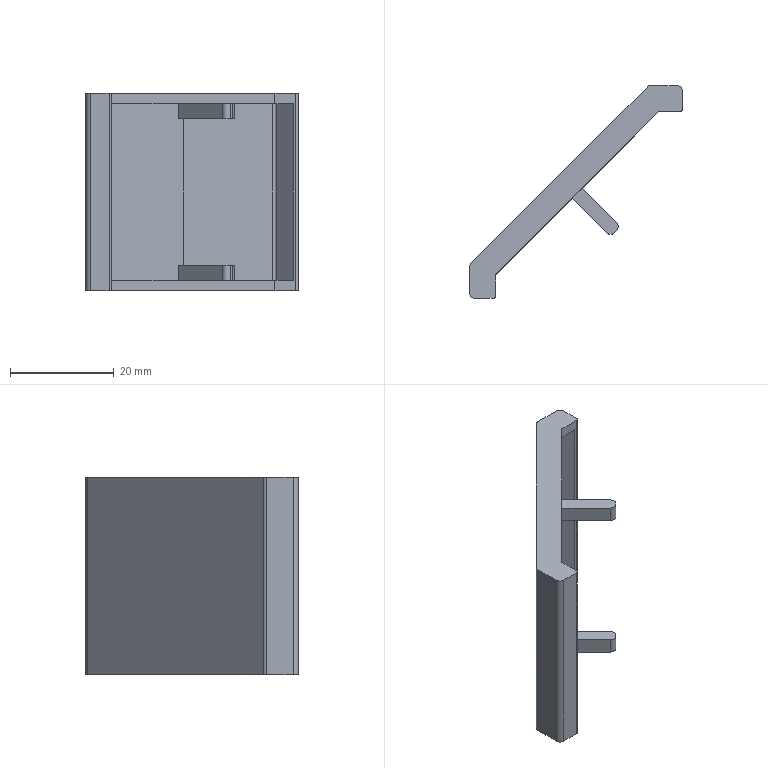Part | SolidWorks | features BaseBody 1 | 1 solid | 42 faces | box 41 x 41 x 38 mm | volume 6489 mm3 | plane 29 | cylinder 13 | commonest cylinder face diameters 2 x9 1 x4
STEP:
#1=CARTESIAN_POINT('',(11.11,-10.616,-17.));
#2=VERTEX_POINT('',#1);
#3=CARTESIAN_POINT('',(11.403,-9.909,-17.));
#4=VERTEX_POINT('',#3);
#5=CARTESIAN_POINT('',(10.403,-9.909,-17.));
#6=DIRECTION('',(0.,0.,1.));
#7=DIRECTION('',(1.,0.,0.));
#8=AXIS2_PLACEMENT_3D('',#5,#6,#7);
#9=CIRCLE('',#8,1.);
#10=EDGE_CURVE('',#2,#4,#9,.T.);
#11=ORIENTED_EDGE('',*,*,#10,.T.);
#12=CARTESIAN_POINT('',(11.403,-9.909,-14.1));
#13=VERTEX_POINT('',#12);
#14=CARTESIAN_POINT('',(11.403,-9.909,-14.1));
#15=DIRECTION('',(0.,0.,1.));
#16=VECTOR('',#15,1000.);
#17=LINE('',#14,#16);
#18=EDGE_CURVE('',#4,#13,#17,.T.);
#19=ORIENTED_EDGE('',*,*,#18,.T.);
#20=CARTESIAN_POINT('',(11.11,-10.616,-14.1));
#21=VERTEX_POINT('',#20);
#22=CARTESIAN_POINT('',(10.403,-9.909,-14.1));
#23=DIRECTION('',(0.,0.,1.));
#24=DIRECTION('',(1.,0.,0.));
#25=AXIS2_PLACEMENT_3D('',#22,#23,#24);
#26=CIRCLE('',#25,1.);
#27=EDGE_CURVE('',#21,#13,#26,.T.);
#28=ORIENTED_EDGE('',*,*,#27,.F.);
#29=CARTESIAN_POINT('',(11.11,-10.616,-14.1));
#30=DIRECTION('',(0.,0.,-1.));
#31=VECTOR('',#30,1000.);
#32=LINE('',#29,#31);
#33=EDGE_CURVE('',#21,#2,#32,.T.);
#34=ORIENTED_EDGE('',*,*,#33,.T.);
#35=EDGE_LOOP('',(#11,#19,#28,#34));
#36=FACE_OUTER_BOUND('',#35,.T.);
#37=CARTESIAN_POINT('',(10.403,-9.909,-14.1));
#38=DIRECTION('',(0.,0.,1.));
#39=DIRECTION('',(1.,0.,0.));
#40=AXIS2_PLACEMENT_3D('',#37,#38,#39);
#41=CYLINDRICAL_SURFACE('',#40,1.);
#42=ADVANCED_FACE('',(#36),#41,.T.);
#43=CARTESIAN_POINT('',(-16.957,-16.957,19.));
#44=VERTEX_POINT('',#43);
#45=CARTESIAN_POINT('',(-16.957,-16.957,-19.));
#46=VERTEX_POINT('',#45);
#47=CARTESIAN_POINT('',(-16.957,-16.957,19.));
#48=DIRECTION('',(0.,0.,-1.));
#49=VECTOR('',#48,1000.);
#50=LINE('',#47,#49);
#51=EDGE_CURVE('',#44,#46,#50,.T.);
#52=ORIENTED_EDGE('',*,*,#51,.F.);
#53=CARTESIAN_POINT('',(16.957,16.957,19.));
#54=VERTEX_POINT('',#53);
#55=CARTESIAN_POINT('',(16.957,16.957,19.));
#56=DIRECTION('',(-0.7071,-0.7071,0.));
#57=VECTOR('',#56,1000.);
#58=LINE('',#55,#57);
#59=EDGE_CURVE('',#54,#44,#58,.T.);
#60=ORIENTED_EDGE('',*,*,#59,.F.);
#61=CARTESIAN_POINT('',(16.957,16.957,-19.));
#62=VERTEX_POINT('',#61);
#63=CARTESIAN_POINT('',(16.957,16.957,19.));
#64=DIRECTION('',(0.,0.,1.));
#65=VECTOR('',#64,1000.);
#66=LINE('',#63,#65);
#67=EDGE_CURVE('',#62,#54,#66,.T.);
#68=ORIENTED_EDGE('',*,*,#67,.F.);
#69=CARTESIAN_POINT('',(16.957,16.957,-19.));
#70=DIRECTION('',(0.7071,0.7071,0.));
#71=VECTOR('',#70,1000.);
#72=LINE('',#69,#71);
#73=EDGE_CURVE('',#46,#62,#72,.T.);
#74=ORIENTED_EDGE('',*,*,#73,.F.);
#75=EDGE_LOOP('',(#52,#60,#68,#74));
#76=FACE_OUTER_BOUND('',#75,.T.);
#77=CARTESIAN_POINT('',(16.957,16.957,19.));
#78=DIRECTION('',(0.7071,-0.7071,0.));
#79=DIRECTION('',(0.7071,0.7071,0.));
#80=AXIS2_PLACEMENT_3D('',#77,#78,#79);
#81=PLANE('',#80);
#82=ADVANCED_FACE('',(#76),#81,.F.);
#83=CARTESIAN_POINT('',(-17.25,-17.664,-19.));
#84=VERTEX_POINT('',#83);
#85=CARTESIAN_POINT('',(-16.25,-17.664,-19.));
#86=DIRECTION('',(0.,0.,1.));
#87=DIRECTION('',(1.,0.,0.));
#88=AXIS2_PLACEMENT_3D('',#85,#86,#87);
#89=CIRCLE('',#88,1.);
#90=EDGE_CURVE('',#46,#84,#89,.T.);
#91=ORIENTED_EDGE('',*,*,#90,.F.);
#92=ORIENTED_EDGE('',*,*,#73,.T.);
#93=CARTESIAN_POINT('',(17.664,17.25,-19.));
#94=VERTEX_POINT('',#93);
#95=CARTESIAN_POINT('',(17.664,16.25,-19.));
#96=DIRECTION('',(0.,0.,1.));
#97=DIRECTION('',(1.,0.,0.));
#98=AXIS2_PLACEMENT_3D('',#95,#96,#97);
#99=CIRCLE('',#98,1.);
#100=EDGE_CURVE('',#94,#62,#99,.T.);
#101=ORIENTED_EDGE('',*,*,#100,.F.);
#102=CARTESIAN_POINT('',(22.75,17.25,-19.));
#103=VERTEX_POINT('',#102);
#104=CARTESIAN_POINT('',(-16.25,17.25,-19.));
#105=DIRECTION('',(-1.,0.,0.));
#106=VECTOR('',#105,1000.);
#107=LINE('',#104,#106);
#108=EDGE_CURVE('',#103,#94,#107,.T.);
#109=ORIENTED_EDGE('',*,*,#108,.F.);
#110=CARTESIAN_POINT('',(23.75,16.25,-19.));
#111=VERTEX_POINT('',#110);
#112=CARTESIAN_POINT('',(22.75,16.25,-19.));
#113=DIRECTION('',(0.,0.,1.));
#114=DIRECTION('',(1.,0.,0.));
#115=AXIS2_PLACEMENT_3D('',#112,#113,#114);
#116=CIRCLE('',#115,1.);
#117=EDGE_CURVE('',#111,#103,#116,.T.);
#118=ORIENTED_EDGE('',*,*,#117,.F.);
#119=CARTESIAN_POINT('',(23.75,12.75,-19.));
#120=VERTEX_POINT('',#119);
#121=CARTESIAN_POINT('',(23.75,-22.75,-19.));
#122=DIRECTION('',(0.,1.,0.));
#123=VECTOR('',#122,1000.);
#124=LINE('',#121,#123);
#125=EDGE_CURVE('',#120,#111,#124,.T.);
#126=ORIENTED_EDGE('',*,*,#125,.F.);
#127=CARTESIAN_POINT('',(23.25,12.25,-19.));
#128=VERTEX_POINT('',#127);
#129=CARTESIAN_POINT('',(23.25,12.75,-19.));
#130=DIRECTION('',(0.,0.,1.));
#131=DIRECTION('',(1.,0.,0.));
#132=AXIS2_PLACEMENT_3D('',#129,#130,#131);
#133=CIRCLE('',#132,0.5);
#134=EDGE_CURVE('',#128,#120,#133,.T.);
#135=ORIENTED_EDGE('',*,*,#134,.F.);
#136=CARTESIAN_POINT('',(19.25,12.25,-19.));
#137=VERTEX_POINT('',#136);
#138=CARTESIAN_POINT('',(-16.25,12.25,-19.));
#139=DIRECTION('',(1.,0.,0.));
#140=VECTOR('',#139,1000.);
#141=LINE('',#138,#140);
#142=EDGE_CURVE('',#137,#128,#141,.T.);
#143=ORIENTED_EDGE('',*,*,#142,.F.);
#144=CARTESIAN_POINT('',(-12.25,-19.25,-19.));
#145=VERTEX_POINT('',#144);
#146=CARTESIAN_POINT('',(-12.25,-19.25,-19.));
#147=DIRECTION('',(0.7071,0.7071,0.));
#148=VECTOR('',#147,1000.);
#149=LINE('',#146,#148);
#150=EDGE_CURVE('',#145,#137,#149,.T.);
#151=ORIENTED_EDGE('',*,*,#150,.F.);
#152=CARTESIAN_POINT('',(-12.25,-23.25,-19.));
#153=VERTEX_POINT('',#152);
#154=CARTESIAN_POINT('',(-12.25,-22.75,-19.));
#155=DIRECTION('',(0.,1.,0.));
#156=VECTOR('',#155,1000.);
#157=LINE('',#154,#156);
#158=EDGE_CURVE('',#153,#145,#157,.T.);
#159=ORIENTED_EDGE('',*,*,#158,.F.);
#160=CARTESIAN_POINT('',(-12.75,-23.75,-19.));
#161=VERTEX_POINT('',#160);
#162=CARTESIAN_POINT('',(-12.75,-23.25,-19.));
#163=DIRECTION('',(0.,0.,1.));
#164=DIRECTION('',(1.,0.,0.));
#165=AXIS2_PLACEMENT_3D('',#162,#163,#164);
#166=CIRCLE('',#165,0.5);
#167=EDGE_CURVE('',#161,#153,#166,.T.);
#168=ORIENTED_EDGE('',*,*,#167,.F.);
#169=CARTESIAN_POINT('',(-16.25,-23.75,-19.));
#170=VERTEX_POINT('',#169);
#171=CARTESIAN_POINT('',(-16.25,-23.75,-19.));
#172=DIRECTION('',(1.,0.,0.));
#173=VECTOR('',#172,1000.);
#174=LINE('',#171,#173);
#175=EDGE_CURVE('',#170,#161,#174,.T.);
#176=ORIENTED_EDGE('',*,*,#175,.F.);
#177=CARTESIAN_POINT('',(-17.25,-22.75,-19.));
#178=VERTEX_POINT('',#177);
#179=CARTESIAN_POINT('',(-16.25,-22.75,-19.));
#180=DIRECTION('',(0.,0.,1.));
#181=DIRECTION('',(1.,0.,0.));
#182=AXIS2_PLACEMENT_3D('',#179,#180,#181);
#183=CIRCLE('',#182,1.);
#184=EDGE_CURVE('',#178,#170,#183,.T.);
#185=ORIENTED_EDGE('',*,*,#184,.F.);
#186=CARTESIAN_POINT('',(-17.25,-22.75,-19.));
#187=DIRECTION('',(0.,-1.,0.));
#188=VECTOR('',#187,1000.);
#189=LINE('',#186,#188);
#190=EDGE_CURVE('',#84,#178,#189,.T.);
#191=ORIENTED_EDGE('',*,*,#190,.F.);
#192=EDGE_LOOP('',(#91,#92,#101,#109,#118,#126,#135,#143,#151,#159,#168,#176,#185,#191));
#193=FACE_OUTER_BOUND('',#192,.T.);
#194=CARTESIAN_POINT('',(-16.25,-22.75,-19.));
#195=DIRECTION('',(0.,0.,1.));
#196=DIRECTION('',(1.,0.,0.));
#197=AXIS2_PLACEMENT_3D('',#194,#195,#196);
#198=PLANE('',#197);
#199=ADVANCED_FACE('',(#193),#198,.F.);
#200=CARTESIAN_POINT('',(-17.25,-17.664,19.));
#201=VERTEX_POINT('',#200);
#202=CARTESIAN_POINT('',(-16.25,-17.664,19.));
#203=DIRECTION('',(0.,0.,-1.));
#204=DIRECTION('',(1.,0.,0.));
#205=AXIS2_PLACEMENT_3D('',#202,#203,#204);
#206=CIRCLE('',#205,1.);
#207=EDGE_CURVE('',#201,#44,#206,.T.);
#208=ORIENTED_EDGE('',*,*,#207,.T.);
#209=ORIENTED_EDGE('',*,*,#51,.T.);
#210=ORIENTED_EDGE('',*,*,#90,.T.);
#211=CARTESIAN_POINT('',(-17.25,-17.664,19.));
#212=DIRECTION('',(0.,0.,1.));
#213=VECTOR('',#212,1000.);
#214=LINE('',#211,#213);
#215=EDGE_CURVE('',#84,#201,#214,.T.);
#216=ORIENTED_EDGE('',*,*,#215,.T.);
#217=EDGE_LOOP('',(#208,#209,#210,#216));
#218=FACE_OUTER_BOUND('',#217,.T.);
#219=CARTESIAN_POINT('',(-16.25,-17.664,19.));
#220=DIRECTION('',(0.,0.,1.));
#221=DIRECTION('',(1.,0.,0.));
#222=AXIS2_PLACEMENT_3D('',#219,#220,#221);
#223=CYLINDRICAL_SURFACE('',#222,1.);
#224=ADVANCED_FACE('',(#218),#223,.T.);
#225=ORIENTED_EDGE('',*,*,#59,.T.);
#226=ORIENTED_EDGE('',*,*,#207,.F.);
#227=CARTESIAN_POINT('',(-17.25,-22.75,19.));
#228=VERTEX_POINT('',#227);
#229=CARTESIAN_POINT('',(-17.25,-22.75,19.));
#230=DIRECTION('',(0.,-1.,0.));
#231=VECTOR('',#230,1000.);
#232=LINE('',#229,#231);
#233=EDGE_CURVE('',#201,#228,#232,.T.);
#234=ORIENTED_EDGE('',*,*,#233,.T.);
#235=CARTESIAN_POINT('',(-16.25,-23.75,19.));
#236=VERTEX_POINT('',#235);
#237=CARTESIAN_POINT('',(-16.25,-22.75,19.));
#238=DIRECTION('',(0.,0.,-1.));
#239=DIRECTION('',(1.,0.,0.));
#240=AXIS2_PLACEMENT_3D('',#237,#238,#239);
#241=CIRCLE('',#240,1.);
#242=EDGE_CURVE('',#236,#228,#241,.T.);
#243=ORIENTED_EDGE('',*,*,#242,.F.);
#244=CARTESIAN_POINT('',(-12.75,-23.75,19.));
#245=VERTEX_POINT('',#244);
#246=CARTESIAN_POINT('',(-16.25,-23.75,19.));
#247=DIRECTION('',(1.,0.,0.));
#248=VECTOR('',#247,1000.);
#249=LINE('',#246,#248);
#250=EDGE_CURVE('',#236,#245,#249,.T.);
#251=ORIENTED_EDGE('',*,*,#250,.T.);
#252=CARTESIAN_POINT('',(-12.25,-23.25,19.));
#253=VERTEX_POINT('',#252);
#254=CARTESIAN_POINT('',(-12.75,-23.25,19.));
#255=DIRECTION('',(0.,0.,-1.));
#256=DIRECTION('',(1.,0.,0.));
#257=AXIS2_PLACEMENT_3D('',#254,#255,#256);
#258=CIRCLE('',#257,0.5);
#259=EDGE_CURVE('',#253,#245,#258,.T.);
#260=ORIENTED_EDGE('',*,*,#259,.F.);
#261=CARTESIAN_POINT('',(-12.25,-19.25,19.));
#262=VERTEX_POINT('',#261);
#263=CARTESIAN_POINT('',(-12.25,-22.75,19.));
#264=DIRECTION('',(0.,1.,0.));
#265=VECTOR('',#264,1000.);
#266=LINE('',#263,#265);
#267=EDGE_CURVE('',#253,#262,#266,.T.);
#268=ORIENTED_EDGE('',*,*,#267,.T.);
#269=CARTESIAN_POINT('',(19.25,12.25,19.));
#270=VERTEX_POINT('',#269);
#271=CARTESIAN_POINT('',(-12.25,-19.25,19.));
#272=DIRECTION('',(0.7071,0.7071,0.));
#273=VECTOR('',#272,1000.);
#274=LINE('',#271,#273);
#275=EDGE_CURVE('',#262,#270,#274,.T.);
#276=ORIENTED_EDGE('',*,*,#275,.T.);
#277=CARTESIAN_POINT('',(23.25,12.25,19.));
#278=VERTEX_POINT('',#277);
#279=CARTESIAN_POINT('',(-16.25,12.25,19.));
#280=DIRECTION('',(1.,0.,0.));
#281=VECTOR('',#280,1000.);
#282=LINE('',#279,#281);
#283=EDGE_CURVE('',#270,#278,#282,.T.);
#284=ORIENTED_EDGE('',*,*,#283,.T.);
#285=CARTESIAN_POINT('',(23.75,12.75,19.));
#286=VERTEX_POINT('',#285);
#287=CARTESIAN_POINT('',(23.25,12.75,19.));
#288=DIRECTION('',(0.,0.,-1.));
#289=DIRECTION('',(1.,0.,0.));
#290=AXIS2_PLACEMENT_3D('',#287,#288,#289);
#291=CIRCLE('',#290,0.5);
#292=EDGE_CURVE('',#286,#278,#291,.T.);
#293=ORIENTED_EDGE('',*,*,#292,.F.);
#294=CARTESIAN_POINT('',(23.75,16.25,19.));
#295=VERTEX_POINT('',#294);
#296=CARTESIAN_POINT('',(23.75,-22.75,19.));
#297=DIRECTION('',(0.,1.,0.));
#298=VECTOR('',#297,1000.);
#299=LINE('',#296,#298);
#300=EDGE_CURVE('',#286,#295,#299,.T.);
#301=ORIENTED_EDGE('',*,*,#300,.T.);
#302=CARTESIAN_POINT('',(22.75,17.25,19.));
#303=VERTEX_POINT('',#302);
#304=CARTESIAN_POINT('',(22.75,16.25,19.));
#305=DIRECTION('',(0.,0.,-1.));
#306=DIRECTION('',(1.,0.,0.));
#307=AXIS2_PLACEMENT_3D('',#304,#305,#306);
#308=CIRCLE('',#307,1.);
#309=EDGE_CURVE('',#303,#295,#308,.T.);
#310=ORIENTED_EDGE('',*,*,#309,.F.);
#311=CARTESIAN_POINT('',(17.664,17.25,19.));
#312=VERTEX_POINT('',#311);
#313=CARTESIAN_POINT('',(-16.25,17.25,19.));
#314=DIRECTION('',(-1.,0.,0.));
#315=VECTOR('',#314,1000.);
#316=LINE('',#313,#315);
#317=EDGE_CURVE('',#303,#312,#316,.T.);
#318=ORIENTED_EDGE('',*,*,#317,.T.);
#319=CARTESIAN_POINT('',(17.664,16.25,19.));
#320=DIRECTION('',(0.,0.,1.));
#321=DIRECTION('',(1.,0.,0.));
#322=AXIS2_PLACEMENT_3D('',#319,#320,#321);
#323=CIRCLE('',#322,1.);
#324=EDGE_CURVE('',#312,#54,#323,.T.);
#325=ORIENTED_EDGE('',*,*,#324,.T.);
#326=EDGE_LOOP('',(#225,#226,#234,#243,#251,#260,#268,#276,#284,#293,#301,#310,#318,#325));
#327=FACE_OUTER_BOUND('',#326,.T.);
#328=CARTESIAN_POINT('',(-16.25,-22.75,19.));
#329=DIRECTION('',(0.,0.,1.));
#330=DIRECTION('',(1.,0.,0.));
#331=AXIS2_PLACEMENT_3D('',#328,#329,#330);
#332=PLANE('',#331);
#333=ADVANCED_FACE('',(#327),#332,.T.);
#334=ORIENTED_EDGE('',*,*,#324,.F.);
#335=CARTESIAN_POINT('',(17.664,17.25,19.));
#336=DIRECTION('',(0.,0.,-1.));
#337=VECTOR('',#336,1000.);
#338=LINE('',#335,#337);
#339=EDGE_CURVE('',#312,#94,#338,.T.);
#340=ORIENTED_EDGE('',*,*,#339,.T.);
#341=ORIENTED_EDGE('',*,*,#100,.T.);
#342=ORIENTED_EDGE('',*,*,#67,.T.);
#343=EDGE_LOOP('',(#334,#340,#341,#342));
#344=FACE_OUTER_BOUND('',#343,.T.);
#345=CARTESIAN_POINT('',(17.664,16.25,19.));
#346=DIRECTION('',(0.,0.,1.));
#347=DIRECTION('',(1.,0.,0.));
#348=AXIS2_PLACEMENT_3D('',#345,#346,#347);
#349=CYLINDRICAL_SURFACE('',#348,1.);
#350=ADVANCED_FACE('',(#344),#349,.T.);
#351=CARTESIAN_POINT('',(-17.25,-22.75,19.));
#352=DIRECTION('',(0.,0.,-1.));
#353=VECTOR('',#352,1000.);
#354=LINE('',#351,#353);
#355=EDGE_CURVE('',#228,#178,#354,.T.);
#356=ORIENTED_EDGE('',*,*,#355,.F.);
#357=ORIENTED_EDGE('',*,*,#233,.F.);
#358=ORIENTED_EDGE('',*,*,#215,.F.);
#359=ORIENTED_EDGE('',*,*,#190,.T.);
#360=EDGE_LOOP('',(#356,#357,#358,#359));
#361=FACE_OUTER_BOUND('',#360,.T.);
#362=CARTESIAN_POINT('',(-17.25,-17.664,19.));
#363=DIRECTION('',(1.,0.,0.));
#364=DIRECTION('',(0.,0.,-1.));
#365=AXIS2_PLACEMENT_3D('',#362,#363,#364);
#366=PLANE('',#365);
#367=ADVANCED_FACE('',(#361),#366,.F.);
#368=ORIENTED_EDGE('',*,*,#339,.F.);
#369=ORIENTED_EDGE('',*,*,#317,.F.);
#370=CARTESIAN_POINT('',(22.75,17.25,19.));
#371=DIRECTION('',(0.,0.,1.));
#372=VECTOR('',#371,1000.);
#373=LINE('',#370,#372);
#374=EDGE_CURVE('',#103,#303,#373,.T.);
#375=ORIENTED_EDGE('',*,*,#374,.F.);
#376=ORIENTED_EDGE('',*,*,#108,.T.);
#377=EDGE_LOOP('',(#368,#369,#375,#376));
#378=FACE_OUTER_BOUND('',#377,.T.);
#379=CARTESIAN_POINT('',(22.75,17.25,19.));
#380=DIRECTION('',(0.,-1.,0.));
#381=DIRECTION('',(0.,0.,-1.));
#382=AXIS2_PLACEMENT_3D('',#379,#380,#381);
#383=PLANE('',#382);
#384=ADVANCED_FACE('',(#378),#383,.F.);
#385=CARTESIAN_POINT('',(23.75,16.25,19.));
#386=DIRECTION('',(0.,0.,-1.));
#387=VECTOR('',#386,1000.);
#388=LINE('',#385,#387);
#389=EDGE_CURVE('',#295,#111,#388,.T.);
#390=ORIENTED_EDGE('',*,*,#389,.F.);
#391=ORIENTED_EDGE('',*,*,#300,.F.);
#392=CARTESIAN_POINT('',(23.75,12.75,19.));
#393=DIRECTION('',(0.,0.,1.));
#394=VECTOR('',#393,1000.);
#395=LINE('',#392,#394);
#396=EDGE_CURVE('',#120,#286,#395,.T.);
#397=ORIENTED_EDGE('',*,*,#396,.F.);
#398=ORIENTED_EDGE('',*,*,#125,.T.);
#399=EDGE_LOOP('',(#390,#391,#397,#398));
#400=FACE_OUTER_BOUND('',#399,.T.);
#401=CARTESIAN_POINT('',(23.75,12.75,19.));
#402=DIRECTION('',(-1.,0.,0.));
#403=DIRECTION('',(0.,0.,1.));
#404=AXIS2_PLACEMENT_3D('',#401,#402,#403);
#405=PLANE('',#404);
#406=ADVANCED_FACE('',(#400),#405,.F.);
#407=CARTESIAN_POINT('',(22.752,12.25,17.));
#408=VERTEX_POINT('',#407);
#409=CARTESIAN_POINT('',(19.25,12.25,17.));
#410=VERTEX_POINT('',#409);
#411=CARTESIAN_POINT('',(19.25,12.25,17.));
#412=DIRECTION('',(-1.,0.,0.));
#413=VECTOR('',#412,1000.);
#414=LINE('',#411,#413);
#415=EDGE_CURVE('',#408,#410,#414,.T.);
#416=ORIENTED_EDGE('',*,*,#415,.F.);
#417=CARTESIAN_POINT('',(22.752,12.25,-17.));
#418=VERTEX_POINT('',#417);
#419=CARTESIAN_POINT('',(22.752,12.25,19.));
#420=DIRECTION('',(0.,0.,1.));
#421=VECTOR('',#420,1000.);
#422=LINE('',#419,#421);
#423=EDGE_CURVE('',#418,#408,#422,.T.);
#424=ORIENTED_EDGE('',*,*,#423,.F.);
#425=CARTESIAN_POINT('',(19.25,12.25,-17.));
#426=VERTEX_POINT('',#425);
#427=CARTESIAN_POINT('',(19.25,12.25,-17.));
#428=DIRECTION('',(1.,0.,0.));
#429=VECTOR('',#428,1000.);
#430=LINE('',#427,#429);
#431=EDGE_CURVE('',#426,#418,#430,.T.);
#432=ORIENTED_EDGE('',*,*,#431,.F.);
#433=CARTESIAN_POINT('',(19.25,12.25,19.));
#434=DIRECTION('',(0.,0.,1.));
#435=VECTOR('',#434,1000.);
#436=LINE('',#433,#435);
#437=EDGE_CURVE('',#137,#426,#436,.T.);
#438=ORIENTED_EDGE('',*,*,#437,.F.);
#439=ORIENTED_EDGE('',*,*,#142,.T.);
#440=CARTESIAN_POINT('',(23.25,12.25,19.));
#441=DIRECTION('',(0.,0.,-1.));
#442=VECTOR('',#441,1000.);
#443=LINE('',#440,#442);
#444=EDGE_CURVE('',#278,#128,#443,.T.);
#445=ORIENTED_EDGE('',*,*,#444,.F.);
#446=ORIENTED_EDGE('',*,*,#283,.F.);
#447=CARTESIAN_POINT('',(19.25,12.25,19.));
#448=DIRECTION('',(0.,0.,1.));
#449=VECTOR('',#448,1000.);
#450=LINE('',#447,#449);
#451=EDGE_CURVE('',#410,#270,#450,.T.);
#452=ORIENTED_EDGE('',*,*,#451,.F.);
#453=EDGE_LOOP('',(#416,#424,#432,#438,#439,#445,#446,#452));
#454=FACE_OUTER_BOUND('',#453,.T.);
#455=CARTESIAN_POINT('',(19.25,12.25,19.));
#456=DIRECTION('',(0.,1.,0.));
#457=DIRECTION('',(0.,0.,1.));
#458=AXIS2_PLACEMENT_3D('',#455,#456,#457);
#459=PLANE('',#458);
#460=ADVANCED_FACE('',(#454),#459,.F.);
#461=CARTESIAN_POINT('',(-12.25,-19.25,-17.));
#462=VERTEX_POINT('',#461);
#463=CARTESIAN_POINT('',(-12.25,-19.25,19.));
#464=DIRECTION('',(0.,0.,1.));
#465=VECTOR('',#464,1000.);
#466=LINE('',#463,#465);
#467=EDGE_CURVE('',#145,#462,#466,.T.);
#468=ORIENTED_EDGE('',*,*,#467,.F.);
#469=ORIENTED_EDGE('',*,*,#150,.T.);
#470=ORIENTED_EDGE('',*,*,#437,.T.);
#471=CARTESIAN_POINT('',(4.455,-2.545,-17.));
#472=VERTEX_POINT('',#471);
#473=CARTESIAN_POINT('',(-12.25,-19.25,-17.));
#474=DIRECTION('',(0.7071,0.7071,0.));
#475=VECTOR('',#474,1000.);
#476=LINE('',#473,#475);
#477=EDGE_CURVE('',#472,#426,#476,.T.);
#478=ORIENTED_EDGE('',*,*,#477,.F.);
#479=CARTESIAN_POINT('',(2.545,-4.455,-17.));
#480=VERTEX_POINT('',#479);
#481=CARTESIAN_POINT('',(-12.25,-19.25,-17.));
#482=DIRECTION('',(0.7071,0.7071,0.));
#483=VECTOR('',#482,1000.);
#484=LINE('',#481,#483);
#485=EDGE_CURVE('',#480,#472,#484,.T.);
#486=ORIENTED_EDGE('',*,*,#485,.F.);
#487=CARTESIAN_POINT('',(-12.25,-19.25,-17.));
#488=DIRECTION('',(0.7071,0.7071,0.));
#489=VECTOR('',#488,1000.);
#490=LINE('',#487,#489);
#491=EDGE_CURVE('',#462,#480,#490,.T.);
#492=ORIENTED_EDGE('',*,*,#491,.F.);
#493=EDGE_LOOP('',(#468,#469,#470,#478,#486,#492));
#494=FACE_OUTER_BOUND('',#493,.T.);
#495=CARTESIAN_POINT('',(-12.25,-19.25,19.));
#496=DIRECTION('',(-0.7071,0.7071,0.));
#497=DIRECTION('',(-0.7071,-0.7071,0.));
#498=AXIS2_PLACEMENT_3D('',#495,#496,#497);
#499=PLANE('',#498);
#500=ADVANCED_FACE('',(#494),#499,.F.);
#501=CARTESIAN_POINT('',(-12.25,-19.25,17.));
#502=VERTEX_POINT('',#501);
#503=CARTESIAN_POINT('',(-12.25,-22.752,17.));
#504=VERTEX_POINT('',#503);
#505=CARTESIAN_POINT('',(-12.25,-23.25,17.));
#506=DIRECTION('',(0.,-1.,0.));
#507=VECTOR('',#506,1000.);
#508=LINE('',#505,#507);
#509=EDGE_CURVE('',#502,#504,#508,.T.);
#510=ORIENTED_EDGE('',*,*,#509,.F.);
#511=CARTESIAN_POINT('',(-12.25,-19.25,19.));
#512=DIRECTION('',(0.,0.,-1.));
#513=VECTOR('',#512,1000.);
#514=LINE('',#511,#513);
#515=EDGE_CURVE('',#262,#502,#514,.T.);
#516=ORIENTED_EDGE('',*,*,#515,.F.);
#517=ORIENTED_EDGE('',*,*,#267,.F.);
#518=CARTESIAN_POINT('',(-12.25,-23.25,19.));
#519=DIRECTION('',(0.,0.,1.));
#520=VECTOR('',#519,1000.);
#521=LINE('',#518,#520);
#522=EDGE_CURVE('',#153,#253,#521,.T.);
#523=ORIENTED_EDGE('',*,*,#522,.F.);
#524=ORIENTED_EDGE('',*,*,#158,.T.);
#525=ORIENTED_EDGE('',*,*,#467,.T.);
#526=CARTESIAN_POINT('',(-12.25,-22.752,-17.));
#527=VERTEX_POINT('',#526);
#528=CARTESIAN_POINT('',(-12.25,-23.25,-17.));
#529=DIRECTION('',(0.,1.,0.));
#530=VECTOR('',#529,1000.);
#531=LINE('',#528,#530);
#532=EDGE_CURVE('',#527,#462,#531,.T.);
#533=ORIENTED_EDGE('',*,*,#532,.F.);
#534=CARTESIAN_POINT('',(-12.25,-22.752,19.));
#535=DIRECTION('',(0.,0.,-1.));
#536=VECTOR('',#535,1000.);
#537=LINE('',#534,#536);
#538=EDGE_CURVE('',#504,#527,#537,.T.);
#539=ORIENTED_EDGE('',*,*,#538,.F.);
#540=EDGE_LOOP('',(#510,#516,#517,#523,#524,#525,#533,#539));
#541=FACE_OUTER_BOUND('',#540,.T.);
#542=CARTESIAN_POINT('',(-12.25,-23.25,19.));
#543=DIRECTION('',(-1.,0.,0.));
#544=DIRECTION('',(0.,0.,1.));
#545=AXIS2_PLACEMENT_3D('',#542,#543,#544);
#546=PLANE('',#545);
#547=ADVANCED_FACE('',(#541),#546,.F.);
#548=CARTESIAN_POINT('',(-12.75,-23.75,19.));
#549=DIRECTION('',(0.,0.,-1.));
#550=VECTOR('',#549,1000.);
#551=LINE('',#548,#550);
#552=EDGE_CURVE('',#245,#161,#551,.T.);
#553=ORIENTED_EDGE('',*,*,#552,.F.);
#554=ORIENTED_EDGE('',*,*,#250,.F.);
#555=CARTESIAN_POINT('',(-16.25,-23.75,19.));
#556=DIRECTION('',(0.,0.,1.));
#557=VECTOR('',#556,1000.);
#558=LINE('',#555,#557);
#559=EDGE_CURVE('',#170,#236,#558,.T.);
#560=ORIENTED_EDGE('',*,*,#559,.F.);
#561=ORIENTED_EDGE('',*,*,#175,.T.);
#562=EDGE_LOOP('',(#553,#554,#560,#561));
#563=FACE_OUTER_BOUND('',#562,.T.);
#564=CARTESIAN_POINT('',(-16.25,-23.75,19.));
#565=DIRECTION('',(0.,1.,0.));
#566=DIRECTION('',(0.,0.,1.));
#567=AXIS2_PLACEMENT_3D('',#564,#565,#566);
#568=PLANE('',#567);
#569=ADVANCED_FACE('',(#563),#568,.F.);
#570=CARTESIAN_POINT('',(2.545,-4.455,17.));
#571=VERTEX_POINT('',#570);
#572=CARTESIAN_POINT('',(-12.25,-19.25,17.));
#573=DIRECTION('',(-0.7071,-0.7071,0.));
#574=VECTOR('',#573,1000.);
#575=LINE('',#572,#574);
#576=EDGE_CURVE('',#571,#502,#575,.T.);
#577=ORIENTED_EDGE('',*,*,#576,.F.);
#578=CARTESIAN_POINT('',(4.455,-2.545,17.));
#579=VERTEX_POINT('',#578);
#580=CARTESIAN_POINT('',(-12.25,-19.25,17.));
#581=DIRECTION('',(-0.7071,-0.7071,0.));
#582=VECTOR('',#581,1000.);
#583=LINE('',#580,#582);
#584=EDGE_CURVE('',#579,#571,#583,.T.);
#585=ORIENTED_EDGE('',*,*,#584,.F.);
#586=CARTESIAN_POINT('',(-12.25,-19.25,17.));
#587=DIRECTION('',(-0.7071,-0.7071,0.));
#588=VECTOR('',#587,1000.);
#589=LINE('',#586,#588);
#590=EDGE_CURVE('',#410,#579,#589,.T.);
#591=ORIENTED_EDGE('',*,*,#590,.F.);
#592=ORIENTED_EDGE('',*,*,#451,.T.);
#593=ORIENTED_EDGE('',*,*,#275,.F.);
#594=ORIENTED_EDGE('',*,*,#515,.T.);
#595=EDGE_LOOP('',(#577,#585,#591,#592,#593,#594));
#596=FACE_OUTER_BOUND('',#595,.T.);
#597=CARTESIAN_POINT('',(-12.25,-19.25,19.));
#598=DIRECTION('',(-0.7071,0.7071,0.));
#599=DIRECTION('',(-0.7071,-0.7071,0.));
#600=AXIS2_PLACEMENT_3D('',#597,#598,#599);
#601=PLANE('',#600);
#602=ADVANCED_FACE('',(#596),#601,.F.);
#603=ORIENTED_EDGE('',*,*,#242,.T.);
#604=ORIENTED_EDGE('',*,*,#355,.T.);
#605=ORIENTED_EDGE('',*,*,#184,.T.);
#606=ORIENTED_EDGE('',*,*,#559,.T.);
#607=EDGE_LOOP('',(#603,#604,#605,#606));
#608=FACE_OUTER_BOUND('',#607,.T.);
#609=CARTESIAN_POINT('',(-16.25,-22.75,19.));
#610=DIRECTION('',(0.,0.,1.));
#611=DIRECTION('',(1.,0.,0.));
#612=AXIS2_PLACEMENT_3D('',#609,#610,#611);
#613=CYLINDRICAL_SURFACE('',#612,1.);
#614=ADVANCED_FACE('',(#608),#613,.T.);
#615=ORIENTED_EDGE('',*,*,#309,.T.);
#616=ORIENTED_EDGE('',*,*,#389,.T.);
#617=ORIENTED_EDGE('',*,*,#117,.T.);
#618=ORIENTED_EDGE('',*,*,#374,.T.);
#619=EDGE_LOOP('',(#615,#616,#617,#618));
#620=FACE_OUTER_BOUND('',#619,.T.);
#621=CARTESIAN_POINT('',(22.75,16.25,19.));
#622=DIRECTION('',(0.,0.,1.));
#623=DIRECTION('',(1.,0.,0.));
#624=AXIS2_PLACEMENT_3D('',#621,#622,#623);
#625=CYLINDRICAL_SURFACE('',#624,1.);
#626=ADVANCED_FACE('',(#620),#625,.T.);
#627=ORIENTED_EDGE('',*,*,#292,.T.);
#628=ORIENTED_EDGE('',*,*,#444,.T.);
#629=ORIENTED_EDGE('',*,*,#134,.T.);
#630=ORIENTED_EDGE('',*,*,#396,.T.);
#631=EDGE_LOOP('',(#627,#628,#629,#630));
#632=FACE_OUTER_BOUND('',#631,.T.);
#633=CARTESIAN_POINT('',(23.25,12.75,19.));
#634=DIRECTION('',(0.,0.,1.));
#635=DIRECTION('',(1.,0.,0.));
#636=AXIS2_PLACEMENT_3D('',#633,#634,#635);
#637=CYLINDRICAL_SURFACE('',#636,0.5);
#638=ADVANCED_FACE('',(#632),#637,.T.);
#639=CARTESIAN_POINT('',(2.626,-0.7159,17.));
#640=VERTEX_POINT('',#639);
#641=CARTESIAN_POINT('',(2.626,-0.7159,17.));
#642=DIRECTION('',(0.7071,-0.7072,0.));
#643=VECTOR('',#642,1000.);
#644=LINE('',#641,#643);
#645=EDGE_CURVE('',#640,#579,#644,.T.);
#646=ORIENTED_EDGE('',*,*,#645,.F.);
#647=CARTESIAN_POINT('',(18.818,15.476,17.));
#648=VERTEX_POINT('',#647);
#649=CARTESIAN_POINT('',(18.818,15.476,17.));
#650=DIRECTION('',(-0.7071,-0.7071,0.));
#651=VECTOR('',#650,1000.);
#652=LINE('',#649,#651);
#653=EDGE_CURVE('',#648,#640,#652,.T.);
#654=ORIENTED_EDGE('',*,*,#653,.F.);
#655=CARTESIAN_POINT('',(19.526,15.476,17.));
#656=VERTEX_POINT('',#655);
#657=CARTESIAN_POINT('',(19.172,15.122,17.));
#658=DIRECTION('',(0.,0.,-1.));
#659=DIRECTION('',(1.,0.,0.));
#660=AXIS2_PLACEMENT_3D('',#657,#658,#659);
#661=CIRCLE('',#660,0.5);
#662=EDGE_CURVE('',#648,#656,#661,.T.);
#663=ORIENTED_EDGE('',*,*,#662,.T.);
#664=CARTESIAN_POINT('',(22.752,12.25,17.));
#665=DIRECTION('',(-0.7071,0.7071,0.));
#666=VECTOR('',#665,1000.);
#667=LINE('',#664,#666);
#668=EDGE_CURVE('',#408,#656,#667,.T.);
#669=ORIENTED_EDGE('',*,*,#668,.F.);
#670=ORIENTED_EDGE('',*,*,#415,.T.);
#671=ORIENTED_EDGE('',*,*,#590,.T.);
#672=EDGE_LOOP('',(#646,#654,#663,#669,#670,#671));
#673=FACE_OUTER_BOUND('',#672,.T.);
#674=CARTESIAN_POINT('',(-15.123,-19.172,17.));
#675=DIRECTION('',(0.,0.,1.));
#676=DIRECTION('',(1.,0.,0.));
#677=AXIS2_PLACEMENT_3D('',#674,#675,#676);
#678=PLANE('',#677);
#679=ADVANCED_FACE('',(#673),#678,.F.);
#680=CARTESIAN_POINT('',(19.526,15.476,-17.));
#681=VERTEX_POINT('',#680);
#682=CARTESIAN_POINT('',(19.526,15.476,17.));
#683=DIRECTION('',(0.,0.,-1.));
#684=VECTOR('',#683,1000.);
#685=LINE('',#682,#684);
#686=EDGE_CURVE('',#656,#681,#685,.T.);
#687=ORIENTED_EDGE('',*,*,#686,.T.);
#688=CARTESIAN_POINT('',(24.581,10.421,-17.));
#689=DIRECTION('',(0.7071,-0.7071,0.));
#690=VECTOR('',#689,1000.);
#691=LINE('',#688,#690);
#692=EDGE_CURVE('',#681,#418,#691,.T.);
#693=ORIENTED_EDGE('',*,*,#692,.T.);
#694=ORIENTED_EDGE('',*,*,#423,.T.);
#695=ORIENTED_EDGE('',*,*,#668,.T.);
#696=EDGE_LOOP('',(#687,#693,#694,#695));
#697=FACE_OUTER_BOUND('',#696,.T.);
#698=CARTESIAN_POINT('',(24.581,10.421,17.));
#699=DIRECTION('',(-0.7071,-0.7071,0.));
#700=DIRECTION('',(0.7071,-0.7071,0.));
#701=AXIS2_PLACEMENT_3D('',#698,#699,#700);
#702=PLANE('',#701);
#703=ADVANCED_FACE('',(#697),#702,.T.);
#704=ORIENTED_EDGE('',*,*,#692,.F.);
#705=CARTESIAN_POINT('',(18.818,15.476,-17.));
#706=VERTEX_POINT('',#705);
#707=CARTESIAN_POINT('',(19.172,15.122,-17.));
#708=DIRECTION('',(0.,0.,1.));
#709=DIRECTION('',(1.,0.,0.));
#710=AXIS2_PLACEMENT_3D('',#707,#708,#709);
#711=CIRCLE('',#710,0.5);
#712=EDGE_CURVE('',#681,#706,#711,.T.);
#713=ORIENTED_EDGE('',*,*,#712,.T.);
#714=CARTESIAN_POINT('',(2.626,-0.7159,-17.));
#715=VERTEX_POINT('',#714);
#716=CARTESIAN_POINT('',(18.818,15.476,-17.));
#717=DIRECTION('',(-0.7071,-0.7071,0.));
#718=VECTOR('',#717,1000.);
#719=LINE('',#716,#718);
#720=EDGE_CURVE('',#706,#715,#719,.T.);
#721=ORIENTED_EDGE('',*,*,#720,.T.);
#722=CARTESIAN_POINT('',(2.626,-0.7159,-17.));
#723=DIRECTION('',(0.7071,-0.7072,0.));
#724=VECTOR('',#723,1000.);
#725=LINE('',#722,#724);
#726=EDGE_CURVE('',#715,#472,#725,.T.);
#727=ORIENTED_EDGE('',*,*,#726,.T.);
#728=ORIENTED_EDGE('',*,*,#477,.T.);
#729=ORIENTED_EDGE('',*,*,#431,.T.);
#730=EDGE_LOOP('',(#704,#713,#721,#727,#728,#729));
#731=FACE_OUTER_BOUND('',#730,.T.);
#732=CARTESIAN_POINT('',(-15.123,-19.172,-17.));
#733=DIRECTION('',(0.,0.,1.));
#734=DIRECTION('',(1.,0.,0.));
#735=AXIS2_PLACEMENT_3D('',#732,#733,#734);
#736=PLANE('',#735);
#737=ADVANCED_FACE('',(#731),#736,.T.);
#738=CARTESIAN_POINT('',(-15.477,-19.525,-17.));
#739=VERTEX_POINT('',#738);
#740=CARTESIAN_POINT('',(-15.477,-19.525,-17.));
#741=DIRECTION('',(0.7071,-0.7071,0.));
#742=VECTOR('',#741,1000.);
#743=LINE('',#740,#742);
#744=EDGE_CURVE('',#739,#527,#743,.T.);
#745=ORIENTED_EDGE('',*,*,#744,.T.);
#746=ORIENTED_EDGE('',*,*,#532,.T.);
#747=ORIENTED_EDGE('',*,*,#491,.T.);
#748=CARTESIAN_POINT('',(0.716,-2.625,-17.));
#749=VERTEX_POINT('',#748);
#750=CARTESIAN_POINT('',(2.545,-4.455,-17.));
#751=DIRECTION('',(-0.7071,0.7071,0.));
#752=VECTOR('',#751,1000.);
#753=LINE('',#750,#752);
#754=EDGE_CURVE('',#480,#749,#753,.T.);
#755=ORIENTED_EDGE('',*,*,#754,.T.);
#756=CARTESIAN_POINT('',(-15.477,-18.818,-17.));
#757=VERTEX_POINT('',#756);
#758=CARTESIAN_POINT('',(0.716,-2.625,-17.));
#759=DIRECTION('',(-0.7071,-0.7071,0.));
#760=VECTOR('',#759,1000.);
#761=LINE('',#758,#760);
#762=EDGE_CURVE('',#749,#757,#761,.T.);
#763=ORIENTED_EDGE('',*,*,#762,.T.);
#764=CARTESIAN_POINT('',(-15.123,-19.172,-17.));
#765=DIRECTION('',(0.,0.,1.));
#766=DIRECTION('',(1.,0.,0.));
#767=AXIS2_PLACEMENT_3D('',#764,#765,#766);
#768=CIRCLE('',#767,0.5);
#769=EDGE_CURVE('',#757,#739,#768,.T.);
#770=ORIENTED_EDGE('',*,*,#769,.T.);
#771=EDGE_LOOP('',(#745,#746,#747,#755,#763,#770));
#772=FACE_OUTER_BOUND('',#771,.T.);
#773=CARTESIAN_POINT('',(-15.123,-19.172,-17.));
#774=DIRECTION('',(0.,0.,1.));
#775=DIRECTION('',(1.,0.,0.));
#776=AXIS2_PLACEMENT_3D('',#773,#774,#775);
#777=PLANE('',#776);
#778=ADVANCED_FACE('',(#772),#777,.T.);
#779=ORIENTED_EDGE('',*,*,#485,.T.);
#780=CARTESIAN_POINT('',(11.11,-9.202,-17.));
#781=VERTEX_POINT('',#780);
#782=CARTESIAN_POINT('',(11.11,-9.202,-17.));
#783=DIRECTION('',(-0.7071,0.7072,0.));
#784=VECTOR('',#783,1000.);
#785=LINE('',#782,#784);
#786=EDGE_CURVE('',#781,#472,#785,.T.);
#787=ORIENTED_EDGE('',*,*,#786,.F.);
#788=CARTESIAN_POINT('',(10.403,-9.909,-17.));
#789=DIRECTION('',(0.,0.,1.));
#790=DIRECTION('',(1.,0.,0.));
#791=AXIS2_PLACEMENT_3D('',#788,#789,#790);
#792=CIRCLE('',#791,1.);
#793=EDGE_CURVE('',#4,#781,#792,.T.);
#794=ORIENTED_EDGE('',*,*,#793,.F.);
#795=ORIENTED_EDGE('',*,*,#10,.F.);
#796=CARTESIAN_POINT('',(10.616,-11.111,-17.));
#797=VERTEX_POINT('',#796);
#798=CARTESIAN_POINT('',(10.616,-11.111,-17.));
#799=DIRECTION('',(-0.7071,-0.7071,0.));
#800=VECTOR('',#799,1000.);
#801=LINE('',#798,#800);
#802=EDGE_CURVE('',#2,#797,#801,.T.);
#803=ORIENTED_EDGE('',*,*,#802,.T.);
#804=CARTESIAN_POINT('',(9.201,-11.111,-17.));
#805=VERTEX_POINT('',#804);
#806=CARTESIAN_POINT('',(9.909,-10.404,-17.));
#807=DIRECTION('',(0.,0.,1.));
#808=DIRECTION('',(1.,0.,0.));
#809=AXIS2_PLACEMENT_3D('',#806,#807,#808);
#810=CIRCLE('',#809,1.);
#811=EDGE_CURVE('',#805,#797,#810,.T.);
#812=ORIENTED_EDGE('',*,*,#811,.F.);
#813=CARTESIAN_POINT('',(2.545,-4.455,-17.));
#814=DIRECTION('',(0.7071,-0.7071,0.));
#815=VECTOR('',#814,1000.);
#816=LINE('',#813,#815);
#817=EDGE_CURVE('',#480,#805,#816,.T.);
#818=ORIENTED_EDGE('',*,*,#817,.F.);
#819=EDGE_LOOP('',(#779,#787,#794,#795,#803,#812,#818));
#820=FACE_OUTER_BOUND('',#819,.T.);
#821=CARTESIAN_POINT('',(9.909,-10.404,-17.));
#822=DIRECTION('',(0.,0.,1.));
#823=DIRECTION('',(1.,0.,0.));
#824=AXIS2_PLACEMENT_3D('',#821,#822,#823);
#825=PLANE('',#824);
#826=ADVANCED_FACE('',(#820),#825,.F.);
#827=CARTESIAN_POINT('',(-15.477,-19.525,17.));
#828=VERTEX_POINT('',#827);
#829=CARTESIAN_POINT('',(-15.477,-19.525,17.));
#830=DIRECTION('',(0.,0.,1.));
#831=VECTOR('',#830,1000.);
#832=LINE('',#829,#831);
#833=EDGE_CURVE('',#739,#828,#832,.T.);
#834=ORIENTED_EDGE('',*,*,#833,.T.);
#835=CARTESIAN_POINT('',(-15.477,-19.525,17.));
#836=DIRECTION('',(0.7071,-0.7071,0.));
#837=VECTOR('',#836,1000.);
#838=LINE('',#835,#837);
#839=EDGE_CURVE('',#828,#504,#838,.T.);
#840=ORIENTED_EDGE('',*,*,#839,.T.);
#841=ORIENTED_EDGE('',*,*,#538,.T.);
#842=ORIENTED_EDGE('',*,*,#744,.F.);
#843=EDGE_LOOP('',(#834,#840,#841,#842));
#844=FACE_OUTER_BOUND('',#843,.T.);
#845=CARTESIAN_POINT('',(-15.477,-19.525,17.));
#846=DIRECTION('',(0.7071,0.7071,0.));
#847=DIRECTION('',(-0.7071,0.7071,0.));
#848=AXIS2_PLACEMENT_3D('',#845,#846,#847);
#849=PLANE('',#848);
#850=ADVANCED_FACE('',(#844),#849,.T.);
#851=CARTESIAN_POINT('',(0.716,-2.625,17.));
#852=VERTEX_POINT('',#851);
#853=CARTESIAN_POINT('',(2.545,-4.455,17.));
#854=DIRECTION('',(-0.7071,0.7071,0.));
#855=VECTOR('',#854,1000.);
#856=LINE('',#853,#855);
#857=EDGE_CURVE('',#571,#852,#856,.T.);
#858=ORIENTED_EDGE('',*,*,#857,.F.);
#859=ORIENTED_EDGE('',*,*,#576,.T.);
#860=ORIENTED_EDGE('',*,*,#509,.T.);
#861=ORIENTED_EDGE('',*,*,#839,.F.);
#862=CARTESIAN_POINT('',(-15.477,-18.818,17.));
#863=VERTEX_POINT('',#862);
#864=CARTESIAN_POINT('',(-15.123,-19.172,17.));
#865=DIRECTION('',(0.,0.,1.));
#866=DIRECTION('',(1.,0.,0.));
#867=AXIS2_PLACEMENT_3D('',#864,#865,#866);
#868=CIRCLE('',#867,0.5);
#869=EDGE_CURVE('',#863,#828,#868,.T.);
#870=ORIENTED_EDGE('',*,*,#869,.F.);
#871=CARTESIAN_POINT('',(0.716,-2.625,17.));
#872=DIRECTION('',(-0.7071,-0.7071,0.));
#873=VECTOR('',#872,1000.);
#874=LINE('',#871,#873);
#875=EDGE_CURVE('',#852,#863,#874,.T.);
#876=ORIENTED_EDGE('',*,*,#875,.F.);
#877=EDGE_LOOP('',(#858,#859,#860,#861,#870,#876));
#878=FACE_OUTER_BOUND('',#877,.T.);
#879=CARTESIAN_POINT('',(-15.123,-19.172,17.));
#880=DIRECTION('',(0.,0.,1.));
#881=DIRECTION('',(1.,0.,0.));
#882=AXIS2_PLACEMENT_3D('',#879,#880,#881);
#883=PLANE('',#882);
#884=ADVANCED_FACE('',(#878),#883,.F.);
#885=ORIENTED_EDGE('',*,*,#259,.T.);
#886=ORIENTED_EDGE('',*,*,#552,.T.);
#887=ORIENTED_EDGE('',*,*,#167,.T.);
#888=ORIENTED_EDGE('',*,*,#522,.T.);
#889=EDGE_LOOP('',(#885,#886,#887,#888));
#890=FACE_OUTER_BOUND('',#889,.T.);
#891=CARTESIAN_POINT('',(-12.75,-23.25,19.));
#892=DIRECTION('',(0.,0.,1.));
#893=DIRECTION('',(1.,0.,0.));
#894=AXIS2_PLACEMENT_3D('',#891,#892,#893);
#895=CYLINDRICAL_SURFACE('',#894,0.5);
#896=ADVANCED_FACE('',(#890),#895,.T.);
#897=CARTESIAN_POINT('',(11.11,-9.202,17.));
#898=VERTEX_POINT('',#897);
#899=CARTESIAN_POINT('',(11.11,-10.616,17.));
#900=VERTEX_POINT('',#899);
#901=CARTESIAN_POINT('',(10.403,-9.909,17.));
#902=DIRECTION('',(0.,0.,-1.));
#903=DIRECTION('',(-1.,0.,0.));
#904=AXIS2_PLACEMENT_3D('',#901,#902,#903);
#905=CIRCLE('',#904,1.);
#906=EDGE_CURVE('',#898,#900,#905,.T.);
#907=ORIENTED_EDGE('',*,*,#906,.F.);
#908=CARTESIAN_POINT('',(11.11,-9.202,17.));
#909=DIRECTION('',(-0.7071,0.7072,0.));
#910=VECTOR('',#909,1000.);
#911=LINE('',#908,#910);
#912=EDGE_CURVE('',#898,#579,#911,.T.);
#913=ORIENTED_EDGE('',*,*,#912,.T.);
#914=ORIENTED_EDGE('',*,*,#584,.T.);
#915=CARTESIAN_POINT('',(9.201,-11.111,17.));
#916=VERTEX_POINT('',#915);
#917=CARTESIAN_POINT('',(2.545,-4.455,17.));
#918=DIRECTION('',(0.7071,-0.7071,0.));
#919=VECTOR('',#918,1000.);
#920=LINE('',#917,#919);
#921=EDGE_CURVE('',#571,#916,#920,.T.);
#922=ORIENTED_EDGE('',*,*,#921,.T.);
#923=CARTESIAN_POINT('',(10.616,-11.111,17.));
#924=VERTEX_POINT('',#923);
#925=CARTESIAN_POINT('',(9.909,-10.404,17.));
#926=DIRECTION('',(0.,0.,-1.));
#927=DIRECTION('',(-1.,0.,0.));
#928=AXIS2_PLACEMENT_3D('',#925,#926,#927);
#929=CIRCLE('',#928,1.);
#930=EDGE_CURVE('',#924,#916,#929,.T.);
#931=ORIENTED_EDGE('',*,*,#930,.F.);
#932=CARTESIAN_POINT('',(10.616,-11.111,17.));
#933=DIRECTION('',(-0.7071,-0.7071,0.));
#934=VECTOR('',#933,1000.);
#935=LINE('',#932,#934);
#936=EDGE_CURVE('',#900,#924,#935,.T.);
#937=ORIENTED_EDGE('',*,*,#936,.F.);
#938=EDGE_LOOP('',(#907,#913,#914,#922,#931,#937));
#939=FACE_OUTER_BOUND('',#938,.T.);
#940=CARTESIAN_POINT('',(9.909,-10.404,17.));
#941=DIRECTION('',(0.,0.,1.));
#942=DIRECTION('',(1.,0.,0.));
#943=AXIS2_PLACEMENT_3D('',#940,#941,#942);
#944=PLANE('',#943);
#945=ADVANCED_FACE('',(#939),#944,.T.);
#946=ORIENTED_EDGE('',*,*,#912,.F.);
#947=CARTESIAN_POINT('',(11.11,-9.202,14.1));
#948=VERTEX_POINT('',#947);
#949=CARTESIAN_POINT('',(11.11,-9.202,14.1));
#950=DIRECTION('',(0.,0.,-1.));
#951=VECTOR('',#950,1000.);
#952=LINE('',#949,#951);
#953=EDGE_CURVE('',#898,#948,#952,.T.);
#954=ORIENTED_EDGE('',*,*,#953,.T.);
#955=CARTESIAN_POINT('',(2.626,-0.7159,14.1));
#956=VERTEX_POINT('',#955);
#957=CARTESIAN_POINT('',(11.11,-9.202,14.1));
#958=DIRECTION('',(-0.7071,0.7072,0.));
#959=VECTOR('',#958,1000.);
#960=LINE('',#957,#959);
#961=EDGE_CURVE('',#948,#956,#960,.T.);
#962=ORIENTED_EDGE('',*,*,#961,.T.);
#963=CARTESIAN_POINT('',(2.626,-0.7159,14.1));
#964=DIRECTION('',(0.,0.,1.));
#965=VECTOR('',#964,1000.);
#966=LINE('',#963,#965);
#967=EDGE_CURVE('',#956,#640,#966,.T.);
#968=ORIENTED_EDGE('',*,*,#967,.T.);
#969=ORIENTED_EDGE('',*,*,#645,.T.);
#970=EDGE_LOOP('',(#946,#954,#962,#968,#969));
#971=FACE_OUTER_BOUND('',#970,.T.);
#972=CARTESIAN_POINT('',(11.11,-9.202,14.1));
#973=DIRECTION('',(0.7072,0.7071,0.));
#974=DIRECTION('',(-0.7071,0.7072,0.));
#975=AXIS2_PLACEMENT_3D('',#972,#973,#974);
#976=PLANE('',#975);
#977=ADVANCED_FACE('',(#971),#976,.T.);
#978=CARTESIAN_POINT('',(1.671,-1.671,14.1));
#979=VERTEX_POINT('',#978);
#980=CARTESIAN_POINT('',(18.818,15.476,14.1));
#981=DIRECTION('',(-0.7071,-0.7071,0.));
#982=VECTOR('',#981,1000.);
#983=LINE('',#980,#982);
#984=EDGE_CURVE('',#956,#979,#983,.T.);
#985=ORIENTED_EDGE('',*,*,#984,.T.);
#986=CARTESIAN_POINT('',(1.671,-1.671,-14.1));
#987=VERTEX_POINT('',#986);
#988=CARTESIAN_POINT('',(1.671,-1.671,17.));
#989=DIRECTION('',(0.,0.,-1.));
#990=VECTOR('',#989,1000.);
#991=LINE('',#988,#990);
#992=EDGE_CURVE('',#979,#987,#991,.T.);
#993=ORIENTED_EDGE('',*,*,#992,.T.);
#994=CARTESIAN_POINT('',(2.626,-0.7159,-14.1));
#995=VERTEX_POINT('',#994);
#996=CARTESIAN_POINT('',(2.626,-0.7159,-14.1));
#997=DIRECTION('',(-0.7071,-0.7071,0.));
#998=VECTOR('',#997,1000.);
#999=LINE('',#996,#998);
#1000=EDGE_CURVE('',#995,#987,#999,.T.);
#1001=ORIENTED_EDGE('',*,*,#1000,.F.);
#1002=CARTESIAN_POINT('',(2.626,-0.7159,17.));
#1003=DIRECTION('',(0.,0.,-1.));
#1004=VECTOR('',#1003,1000.);
#1005=LINE('',#1002,#1004);
#1006=EDGE_CURVE('',#995,#715,#1005,.T.);
#1007=ORIENTED_EDGE('',*,*,#1006,.T.);
#1008=ORIENTED_EDGE('',*,*,#720,.F.);
#1009=CARTESIAN_POINT('',(18.818,15.476,17.));
#1010=DIRECTION('',(0.,0.,1.));
#1011=VECTOR('',#1010,1000.);
#1012=LINE('',#1009,#1011);
#1013=EDGE_CURVE('',#706,#648,#1012,.T.);
#1014=ORIENTED_EDGE('',*,*,#1013,.T.);
#1015=ORIENTED_EDGE('',*,*,#653,.T.);
#1016=ORIENTED_EDGE('',*,*,#967,.F.);
#1017=EDGE_LOOP('',(#985,#993,#1001,#1007,#1008,#1014,#1015,#1016));
#1018=FACE_OUTER_BOUND('',#1017,.T.);
#1019=CARTESIAN_POINT('',(18.818,15.476,17.));
#1020=DIRECTION('',(0.7071,-0.7071,0.));
#1021=DIRECTION('',(0.7071,0.7071,0.));
#1022=AXIS2_PLACEMENT_3D('',#1019,#1020,#1021);
#1023=PLANE('',#1022);
#1024=ADVANCED_FACE('',(#1018),#1023,.T.);
#1025=ORIENTED_EDGE('',*,*,#686,.F.);
#1026=ORIENTED_EDGE('',*,*,#662,.F.);
#1027=ORIENTED_EDGE('',*,*,#1013,.F.);
#1028=ORIENTED_EDGE('',*,*,#712,.F.);
#1029=EDGE_LOOP('',(#1025,#1026,#1027,#1028));
#1030=FACE_OUTER_BOUND('',#1029,.T.);
#1031=CARTESIAN_POINT('',(19.172,15.122,17.));
#1032=DIRECTION('',(0.,0.,1.));
#1033=DIRECTION('',(1.,0.,0.));
#1034=AXIS2_PLACEMENT_3D('',#1031,#1032,#1033);
#1035=CYLINDRICAL_SURFACE('',#1034,0.5);
#1036=ADVANCED_FACE('',(#1030),#1035,.F.);
#1037=CARTESIAN_POINT('',(11.11,-9.202,-14.1));
#1038=VERTEX_POINT('',#1037);
#1039=CARTESIAN_POINT('',(11.11,-9.202,-14.1));
#1040=DIRECTION('',(-0.7071,0.7072,0.));
#1041=VECTOR('',#1040,1000.);
#1042=LINE('',#1039,#1041);
#1043=EDGE_CURVE('',#1038,#995,#1042,.T.);
#1044=ORIENTED_EDGE('',*,*,#1043,.F.);
#1045=CARTESIAN_POINT('',(11.11,-9.202,-14.1));
#1046=DIRECTION('',(0.,0.,1.));
#1047=VECTOR('',#1046,1000.);
#1048=LINE('',#1045,#1047);
#1049=EDGE_CURVE('',#781,#1038,#1048,.T.);
#1050=ORIENTED_EDGE('',*,*,#1049,.F.);
#1051=ORIENTED_EDGE('',*,*,#786,.T.);
#1052=ORIENTED_EDGE('',*,*,#726,.F.);
#1053=ORIENTED_EDGE('',*,*,#1006,.F.);
#1054=EDGE_LOOP('',(#1044,#1050,#1051,#1052,#1053));
#1055=FACE_OUTER_BOUND('',#1054,.T.);
#1056=CARTESIAN_POINT('',(11.11,-9.202,-14.1));
#1057=DIRECTION('',(-0.7072,-0.7071,0.));
#1058=DIRECTION('',(0.7071,-0.7072,0.));
#1059=AXIS2_PLACEMENT_3D('',#1056,#1057,#1058);
#1060=PLANE('',#1059);
#1061=ADVANCED_FACE('',(#1055),#1060,.F.);
#1062=ORIENTED_EDGE('',*,*,#875,.T.);
#1063=CARTESIAN_POINT('',(-15.477,-18.818,17.));
#1064=DIRECTION('',(0.,0.,-1.));
#1065=VECTOR('',#1064,1000.);
#1066=LINE('',#1063,#1065);
#1067=EDGE_CURVE('',#863,#757,#1066,.T.);
#1068=ORIENTED_EDGE('',*,*,#1067,.T.);
#1069=ORIENTED_EDGE('',*,*,#762,.F.);
#1070=CARTESIAN_POINT('',(0.716,-2.625,-14.1));
#1071=VERTEX_POINT('',#1070);
#1072=CARTESIAN_POINT('',(0.716,-2.625,17.));
#1073=DIRECTION('',(0.,0.,1.));
#1074=VECTOR('',#1073,1000.);
#1075=LINE('',#1072,#1074);
#1076=EDGE_CURVE('',#749,#1071,#1075,.T.);
#1077=ORIENTED_EDGE('',*,*,#1076,.T.);
#1078=CARTESIAN_POINT('',(1.671,-1.671,-14.1));
#1079=DIRECTION('',(0.7071,0.7071,0.));
#1080=VECTOR('',#1079,1000.);
#1081=LINE('',#1078,#1080);
#1082=EDGE_CURVE('',#1071,#987,#1081,.T.);
#1083=ORIENTED_EDGE('',*,*,#1082,.T.);
#1084=ORIENTED_EDGE('',*,*,#992,.F.);
#1085=CARTESIAN_POINT('',(0.716,-2.625,14.1));
#1086=VERTEX_POINT('',#1085);
#1087=CARTESIAN_POINT('',(1.671,-1.671,14.1));
#1088=DIRECTION('',(-0.7071,-0.7071,0.));
#1089=VECTOR('',#1088,1000.);
#1090=LINE('',#1087,#1089);
#1091=EDGE_CURVE('',#979,#1086,#1090,.T.);
#1092=ORIENTED_EDGE('',*,*,#1091,.T.);
#1093=CARTESIAN_POINT('',(0.716,-2.625,17.));
#1094=DIRECTION('',(0.,0.,1.));
#1095=VECTOR('',#1094,1000.);
#1096=LINE('',#1093,#1095);
#1097=EDGE_CURVE('',#1086,#852,#1096,.T.);
#1098=ORIENTED_EDGE('',*,*,#1097,.T.);
#1099=EDGE_LOOP('',(#1062,#1068,#1069,#1077,#1083,#1084,#1092,#1098));
#1100=FACE_OUTER_BOUND('',#1099,.T.);
#1101=CARTESIAN_POINT('',(1.671,-1.671,17.));
#1102=DIRECTION('',(0.7071,-0.7071,0.));
#1103=DIRECTION('',(0.7071,0.7071,0.));
#1104=AXIS2_PLACEMENT_3D('',#1101,#1102,#1103);
#1105=PLANE('',#1104);
#1106=ADVANCED_FACE('',(#1100),#1105,.T.);
#1107=ORIENTED_EDGE('',*,*,#754,.F.);
#1108=ORIENTED_EDGE('',*,*,#817,.T.);
#1109=CARTESIAN_POINT('',(9.201,-11.111,-14.1));
#1110=VERTEX_POINT('',#1109);
#1111=CARTESIAN_POINT('',(9.201,-11.111,-14.1));
#1112=DIRECTION('',(0.,0.,-1.));
#1113=VECTOR('',#1112,1000.);
#1114=LINE('',#1111,#1113);
#1115=EDGE_CURVE('',#1110,#805,#1114,.T.);
#1116=ORIENTED_EDGE('',*,*,#1115,.F.);
#1117=CARTESIAN_POINT('',(0.008893,-1.918,-14.1));
#1118=DIRECTION('',(0.7071,-0.7071,0.));
#1119=VECTOR('',#1118,1000.);
#1120=LINE('',#1117,#1119);
#1121=EDGE_CURVE('',#1071,#1110,#1120,.T.);
#1122=ORIENTED_EDGE('',*,*,#1121,.F.);
#1123=ORIENTED_EDGE('',*,*,#1076,.F.);
#1124=EDGE_LOOP('',(#1107,#1108,#1116,#1122,#1123));
#1125=FACE_OUTER_BOUND('',#1124,.T.);
#1126=CARTESIAN_POINT('',(0.008893,-1.918,-14.1));
#1127=DIRECTION('',(0.7071,0.7071,0.));
#1128=DIRECTION('',(-0.7071,0.7071,0.));
#1129=AXIS2_PLACEMENT_3D('',#1126,#1127,#1128);
#1130=PLANE('',#1129);
#1131=ADVANCED_FACE('',(#1125),#1130,.F.);
#1132=ORIENTED_EDGE('',*,*,#1067,.F.);
#1133=ORIENTED_EDGE('',*,*,#869,.T.);
#1134=ORIENTED_EDGE('',*,*,#833,.F.);
#1135=ORIENTED_EDGE('',*,*,#769,.F.);
#1136=EDGE_LOOP('',(#1132,#1133,#1134,#1135));
#1137=FACE_OUTER_BOUND('',#1136,.T.);
#1138=CARTESIAN_POINT('',(-15.123,-19.172,17.));
#1139=DIRECTION('',(0.,0.,1.));
#1140=DIRECTION('',(1.,0.,0.));
#1141=AXIS2_PLACEMENT_3D('',#1138,#1139,#1140);
#1142=CYLINDRICAL_SURFACE('',#1141,0.5);
#1143=ADVANCED_FACE('',(#1137),#1142,.F.);
#1144=CARTESIAN_POINT('',(9.201,-11.111,14.1));
#1145=VERTEX_POINT('',#1144);
#1146=CARTESIAN_POINT('',(9.201,-11.111,14.1));
#1147=DIRECTION('',(0.,0.,1.));
#1148=VECTOR('',#1147,1000.);
#1149=LINE('',#1146,#1148);
#1150=EDGE_CURVE('',#1145,#916,#1149,.T.);
#1151=ORIENTED_EDGE('',*,*,#1150,.T.);
#1152=ORIENTED_EDGE('',*,*,#921,.F.);
#1153=ORIENTED_EDGE('',*,*,#857,.T.);
#1154=ORIENTED_EDGE('',*,*,#1097,.F.);
#1155=CARTESIAN_POINT('',(0.008893,-1.918,14.1));
#1156=DIRECTION('',(0.7071,-0.7071,0.));
#1157=VECTOR('',#1156,1000.);
#1158=LINE('',#1155,#1157);
#1159=EDGE_CURVE('',#1086,#1145,#1158,.T.);
#1160=ORIENTED_EDGE('',*,*,#1159,.T.);
#1161=EDGE_LOOP('',(#1151,#1152,#1153,#1154,#1160));
#1162=FACE_OUTER_BOUND('',#1161,.T.);
#1163=CARTESIAN_POINT('',(0.008893,-1.918,14.1));
#1164=DIRECTION('',(-0.7071,-0.7071,0.));
#1165=DIRECTION('',(0.7071,-0.7071,0.));
#1166=AXIS2_PLACEMENT_3D('',#1163,#1164,#1165);
#1167=PLANE('',#1166);
#1168=ADVANCED_FACE('',(#1162),#1167,.T.);
#1169=CARTESIAN_POINT('',(11.11,-10.616,14.1));
#1170=VERTEX_POINT('',#1169);
#1171=CARTESIAN_POINT('',(10.403,-9.909,14.1));
#1172=DIRECTION('',(0.,0.,1.));
#1173=DIRECTION('',(-1.,0.,0.));
#1174=AXIS2_PLACEMENT_3D('',#1171,#1172,#1173);
#1175=CIRCLE('',#1174,1.);
#1176=EDGE_CURVE('',#1170,#948,#1175,.T.);
#1177=ORIENTED_EDGE('',*,*,#1176,.T.);
#1178=ORIENTED_EDGE('',*,*,#953,.F.);
#1179=ORIENTED_EDGE('',*,*,#906,.T.);
#1180=CARTESIAN_POINT('',(11.11,-10.616,14.1));
#1181=DIRECTION('',(0.,0.,-1.));
#1182=VECTOR('',#1181,1000.);
#1183=LINE('',#1180,#1182);
#1184=EDGE_CURVE('',#900,#1170,#1183,.T.);
#1185=ORIENTED_EDGE('',*,*,#1184,.T.);
#1186=EDGE_LOOP('',(#1177,#1178,#1179,#1185));
#1187=FACE_OUTER_BOUND('',#1186,.T.);
#1188=CARTESIAN_POINT('',(10.403,-9.909,14.1));
#1189=DIRECTION('',(0.,0.,-1.));
#1190=DIRECTION('',(-1.,0.,0.));
#1191=AXIS2_PLACEMENT_3D('',#1188,#1189,#1190);
#1192=CYLINDRICAL_SURFACE('',#1191,1.);
#1193=ADVANCED_FACE('',(#1187),#1192,.T.);
#1194=ORIENTED_EDGE('',*,*,#984,.F.);
#1195=ORIENTED_EDGE('',*,*,#961,.F.);
#1196=ORIENTED_EDGE('',*,*,#1176,.F.);
#1197=CARTESIAN_POINT('',(10.616,-11.111,14.1));
#1198=VERTEX_POINT('',#1197);
#1199=CARTESIAN_POINT('',(10.616,-11.111,14.1));
#1200=DIRECTION('',(0.7071,0.7071,0.));
#1201=VECTOR('',#1200,1000.);
#1202=LINE('',#1199,#1201);
#1203=EDGE_CURVE('',#1198,#1170,#1202,.T.);
#1204=ORIENTED_EDGE('',*,*,#1203,.F.);
#1205=CARTESIAN_POINT('',(9.909,-10.404,14.1));
#1206=DIRECTION('',(0.,0.,1.));
#1207=DIRECTION('',(-1.,0.,0.));
#1208=AXIS2_PLACEMENT_3D('',#1205,#1206,#1207);
#1209=CIRCLE('',#1208,1.);
#1210=EDGE_CURVE('',#1145,#1198,#1209,.T.);
#1211=ORIENTED_EDGE('',*,*,#1210,.F.);
#1212=ORIENTED_EDGE('',*,*,#1159,.F.);
#1213=ORIENTED_EDGE('',*,*,#1091,.F.);
#1214=EDGE_LOOP('',(#1194,#1195,#1196,#1204,#1211,#1212,#1213));
#1215=FACE_OUTER_BOUND('',#1214,.T.);
#1216=CARTESIAN_POINT('',(9.909,-10.404,14.1));
#1217=DIRECTION('',(0.,0.,1.));
#1218=DIRECTION('',(1.,0.,0.));
#1219=AXIS2_PLACEMENT_3D('',#1216,#1217,#1218);
#1220=PLANE('',#1219);
#1221=ADVANCED_FACE('',(#1215),#1220,.F.);
#1222=ORIENTED_EDGE('',*,*,#27,.T.);
#1223=CARTESIAN_POINT('',(10.403,-9.909,-14.1));
#1224=DIRECTION('',(0.,0.,1.));
#1225=DIRECTION('',(1.,0.,0.));
#1226=AXIS2_PLACEMENT_3D('',#1223,#1224,#1225);
#1227=CIRCLE('',#1226,1.);
#1228=EDGE_CURVE('',#13,#1038,#1227,.T.);
#1229=ORIENTED_EDGE('',*,*,#1228,.T.);
#1230=ORIENTED_EDGE('',*,*,#1043,.T.);
#1231=ORIENTED_EDGE('',*,*,#1000,.T.);
#1232=ORIENTED_EDGE('',*,*,#1082,.F.);
#1233=ORIENTED_EDGE('',*,*,#1121,.T.);
#1234=CARTESIAN_POINT('',(10.616,-11.111,-14.1));
#1235=VERTEX_POINT('',#1234);
#1236=CARTESIAN_POINT('',(9.909,-10.404,-14.1));
#1237=DIRECTION('',(0.,0.,1.));
#1238=DIRECTION('',(1.,0.,0.));
#1239=AXIS2_PLACEMENT_3D('',#1236,#1237,#1238);
#1240=CIRCLE('',#1239,1.);
#1241=EDGE_CURVE('',#1110,#1235,#1240,.T.);
#1242=ORIENTED_EDGE('',*,*,#1241,.T.);
#1243=CARTESIAN_POINT('',(10.616,-11.111,-14.1));
#1244=DIRECTION('',(0.7071,0.7071,0.));
#1245=VECTOR('',#1244,1000.);
#1246=LINE('',#1243,#1245);
#1247=EDGE_CURVE('',#1235,#21,#1246,.T.);
#1248=ORIENTED_EDGE('',*,*,#1247,.T.);
#1249=EDGE_LOOP('',(#1222,#1229,#1230,#1231,#1232,#1233,#1242,#1248));
#1250=FACE_OUTER_BOUND('',#1249,.T.);
#1251=CARTESIAN_POINT('',(9.909,-10.404,-14.1));
#1252=DIRECTION('',(0.,0.,1.));
#1253=DIRECTION('',(1.,0.,0.));
#1254=AXIS2_PLACEMENT_3D('',#1251,#1252,#1253);
#1255=PLANE('',#1254);
#1256=ADVANCED_FACE('',(#1250),#1255,.T.);
#1257=ORIENTED_EDGE('',*,*,#18,.F.);
#1258=ORIENTED_EDGE('',*,*,#793,.T.);
#1259=ORIENTED_EDGE('',*,*,#1049,.T.);
#1260=ORIENTED_EDGE('',*,*,#1228,.F.);
#1261=EDGE_LOOP('',(#1257,#1258,#1259,#1260));
#1262=FACE_OUTER_BOUND('',#1261,.T.);
#1263=CARTESIAN_POINT('',(10.403,-9.909,-14.1));
#1264=DIRECTION('',(0.,0.,1.));
#1265=DIRECTION('',(1.,0.,0.));
#1266=AXIS2_PLACEMENT_3D('',#1263,#1264,#1265);
#1267=CYLINDRICAL_SURFACE('',#1266,1.);
#1268=ADVANCED_FACE('',(#1262),#1267,.T.);
#1269=ORIENTED_EDGE('',*,*,#1241,.F.);
#1270=ORIENTED_EDGE('',*,*,#1115,.T.);
#1271=ORIENTED_EDGE('',*,*,#811,.T.);
#1272=CARTESIAN_POINT('',(10.616,-11.111,-14.1));
#1273=DIRECTION('',(0.,0.,1.));
#1274=VECTOR('',#1273,1000.);
#1275=LINE('',#1272,#1274);
#1276=EDGE_CURVE('',#797,#1235,#1275,.T.);
#1277=ORIENTED_EDGE('',*,*,#1276,.T.);
#1278=EDGE_LOOP('',(#1269,#1270,#1271,#1277));
#1279=FACE_OUTER_BOUND('',#1278,.T.);
#1280=CARTESIAN_POINT('',(9.909,-10.404,-14.1));
#1281=DIRECTION('',(0.,0.,1.));
#1282=DIRECTION('',(1.,0.,0.));
#1283=AXIS2_PLACEMENT_3D('',#1280,#1281,#1282);
#1284=CYLINDRICAL_SURFACE('',#1283,1.);
#1285=ADVANCED_FACE('',(#1279),#1284,.T.);
#1286=ORIENTED_EDGE('',*,*,#1210,.T.);
#1287=CARTESIAN_POINT('',(10.616,-11.111,14.1));
#1288=DIRECTION('',(0.,0.,1.));
#1289=VECTOR('',#1288,1000.);
#1290=LINE('',#1287,#1289);
#1291=EDGE_CURVE('',#1198,#924,#1290,.T.);
#1292=ORIENTED_EDGE('',*,*,#1291,.T.);
#1293=ORIENTED_EDGE('',*,*,#930,.T.);
#1294=ORIENTED_EDGE('',*,*,#1150,.F.);
#1295=EDGE_LOOP('',(#1286,#1292,#1293,#1294));
#1296=FACE_OUTER_BOUND('',#1295,.T.);
#1297=CARTESIAN_POINT('',(9.909,-10.404,14.1));
#1298=DIRECTION('',(0.,0.,-1.));
#1299=DIRECTION('',(-1.,0.,0.));
#1300=AXIS2_PLACEMENT_3D('',#1297,#1298,#1299);
#1301=CYLINDRICAL_SURFACE('',#1300,1.);
#1302=ADVANCED_FACE('',(#1296),#1301,.T.);
#1303=ORIENTED_EDGE('',*,*,#1203,.T.);
#1304=ORIENTED_EDGE('',*,*,#1184,.F.);
#1305=ORIENTED_EDGE('',*,*,#936,.T.);
#1306=ORIENTED_EDGE('',*,*,#1291,.F.);
#1307=EDGE_LOOP('',(#1303,#1304,#1305,#1306));
#1308=FACE_OUTER_BOUND('',#1307,.T.);
#1309=CARTESIAN_POINT('',(10.616,-11.111,14.1));
#1310=DIRECTION('',(0.7071,-0.7071,0.));
#1311=DIRECTION('',(0.7071,0.7071,0.));
#1312=AXIS2_PLACEMENT_3D('',#1309,#1310,#1311);
#1313=PLANE('',#1312);
#1314=ADVANCED_FACE('',(#1308),#1313,.T.);
#1315=ORIENTED_EDGE('',*,*,#33,.F.);
#1316=ORIENTED_EDGE('',*,*,#1247,.F.);
#1317=ORIENTED_EDGE('',*,*,#1276,.F.);
#1318=ORIENTED_EDGE('',*,*,#802,.F.);
#1319=EDGE_LOOP('',(#1315,#1316,#1317,#1318));
#1320=FACE_OUTER_BOUND('',#1319,.T.);
#1321=CARTESIAN_POINT('',(10.616,-11.111,-14.1));
#1322=DIRECTION('',(-0.7071,0.7071,0.));
#1323=DIRECTION('',(-0.7071,-0.7071,0.));
#1324=AXIS2_PLACEMENT_3D('',#1321,#1322,#1323);
#1325=PLANE('',#1324);
#1326=ADVANCED_FACE('',(#1320),#1325,.F.);
#1327=CLOSED_SHELL('',(#42,#82,#199,#224,#333,#350,#367,#384,#406,#460,#500,#547,#569,#602,#614,#626,#638,#679,#703,#737,#778,#826,#850,#884,#896,#945,#977,#1024,#1036,#1061,#1106,#1131,#1143,#1168,#1193,#1221,#1256,#1268,#1285,#1302,#1314,#1326));
#1328=MANIFOLD_SOLID_BREP('',#1327);
#1329=CARTESIAN_POINT('',(0.,0.,0.));
#1330=DIRECTION('',(0.,0.,1.));
#1331=DIRECTION('',(1.,0.,0.));
#1332=AXIS2_PLACEMENT_3D('',#1329,#1330,#1331);
#1333=(LENGTH_UNIT()NAMED_UNIT(*)SI_UNIT(.MILLI.,.METRE.));
#1334=UNCERTAINTY_MEASURE_WITH_UNIT(LENGTH_MEASURE(0.00001),#1333,'','');
#1335=(NAMED_UNIT(*)PLANE_ANGLE_UNIT()SI_UNIT($,.RADIAN.));
#1336=(NAMED_UNIT(*)SI_UNIT($,.STERADIAN.)SOLID_ANGLE_UNIT());
#1337=(GEOMETRIC_REPRESENTATION_CONTEXT(3)GLOBAL_UNCERTAINTY_ASSIGNED_CONTEXT((#1334))GLOBAL_UNIT_ASSIGNED_CONTEXT((#1333,#1335,#1336))REPRESENTATION_CONTEXT('',''));
#1338=ADVANCED_BREP_SHAPE_REPRESENTATION('',(#1328,#1332),#1337);